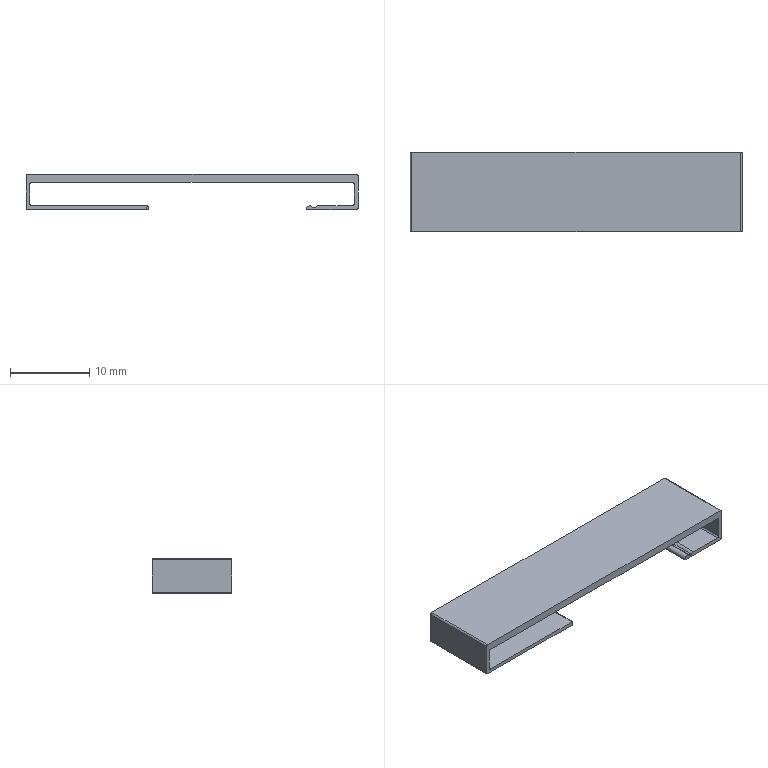Part | SolidWorks | features ICE 4, Extrusion 1, Fillet 1 | 1 solid | 30 faces | box 42 x 10 x 4.5 mm | volume 558.172 mm3 | cylinder 16 | plane 14 | commonest cylinder face diameters 0.4 x12 0.5 x2 0.8 x1 1 x1
STEP:
#1=CARTESIAN_POINT('',(-106.106,120.619,0.2323));
#2=VERTEX_POINT('',#1);
#3=CARTESIAN_POINT('',(-105.914,120.619,0.3216));
#4=VERTEX_POINT('',#3);
#5=CARTESIAN_POINT('',(-106.106,120.619,0.4823));
#6=DIRECTION('',(0.,-1.,0.));
#7=DIRECTION('',(0.,0.,-1.));
#8=AXIS2_PLACEMENT_3D('',#5,#6,#7);
#9=CIRCLE('',#8,0.25);
#10=EDGE_CURVE('',#2,#4,#9,.T.);
#11=ORIENTED_EDGE('',*,*,#10,.F.);
#12=CARTESIAN_POINT('',(-106.106,110.619,0.2323));
#13=VERTEX_POINT('',#12);
#14=CARTESIAN_POINT('',(-106.106,127.138,0.2323));
#15=DIRECTION('',(0.,-1.,0.));
#16=VECTOR('',#15,1000.);
#17=LINE('',#14,#16);
#18=EDGE_CURVE('',#2,#13,#17,.T.);
#19=ORIENTED_EDGE('',*,*,#18,.T.);
#20=CARTESIAN_POINT('',(-105.914,110.619,0.3216));
#21=VERTEX_POINT('',#20);
#22=CARTESIAN_POINT('',(-106.106,110.619,0.4823));
#23=DIRECTION('',(0.,1.,0.));
#24=DIRECTION('',(0.,0.,-1.));
#25=AXIS2_PLACEMENT_3D('',#22,#23,#24);
#26=CIRCLE('',#25,0.25);
#27=EDGE_CURVE('',#21,#13,#26,.T.);
#28=ORIENTED_EDGE('',*,*,#27,.F.);
#29=CARTESIAN_POINT('',(-105.914,127.138,0.3216));
#30=DIRECTION('',(0.,-1.,0.));
#31=VECTOR('',#30,1000.);
#32=LINE('',#29,#31);
#33=EDGE_CURVE('',#4,#21,#32,.T.);
#34=ORIENTED_EDGE('',*,*,#33,.F.);
#35=EDGE_LOOP('',(#11,#19,#28,#34));
#36=FACE_OUTER_BOUND('',#35,.T.);
#37=CARTESIAN_POINT('',(-106.106,127.138,0.4823));
#38=DIRECTION('',(0.,-1.,0.));
#39=DIRECTION('',(0.,0.,-1.));
#40=AXIS2_PLACEMENT_3D('',#37,#38,#39);
#41=CYLINDRICAL_SURFACE('',#40,0.25);
#42=ADVANCED_FACE('',(#36),#41,.F.);
#43=CARTESIAN_POINT('',(-142.531,120.619,4.3));
#44=VERTEX_POINT('',#43);
#45=CARTESIAN_POINT('',(-142.531,120.619,0.2));
#46=VERTEX_POINT('',#45);
#47=CARTESIAN_POINT('',(-142.531,120.619,0.5));
#48=DIRECTION('',(0.,0.,-1.));
#49=VECTOR('',#48,1000.);
#50=LINE('',#47,#49);
#51=EDGE_CURVE('',#44,#46,#50,.T.);
#52=ORIENTED_EDGE('',*,*,#51,.T.);
#53=CARTESIAN_POINT('',(-142.531,110.619,0.2));
#54=VERTEX_POINT('',#53);
#55=CARTESIAN_POINT('',(-142.531,120.619,0.2));
#56=DIRECTION('',(0.,-1.,0.));
#57=VECTOR('',#56,1000.);
#58=LINE('',#55,#57);
#59=EDGE_CURVE('',#46,#54,#58,.T.);
#60=ORIENTED_EDGE('',*,*,#59,.T.);
#61=CARTESIAN_POINT('',(-142.531,110.619,4.3));
#62=VERTEX_POINT('',#61);
#63=CARTESIAN_POINT('',(-142.531,110.619,0.5));
#64=DIRECTION('',(0.,0.,-1.));
#65=VECTOR('',#64,1000.);
#66=LINE('',#63,#65);
#67=EDGE_CURVE('',#62,#54,#66,.T.);
#68=ORIENTED_EDGE('',*,*,#67,.F.);
#69=CARTESIAN_POINT('',(-142.531,120.619,4.3));
#70=DIRECTION('',(0.,1.,0.));
#71=VECTOR('',#70,1000.);
#72=LINE('',#69,#71);
#73=EDGE_CURVE('',#62,#44,#72,.T.);
#74=ORIENTED_EDGE('',*,*,#73,.T.);
#75=EDGE_LOOP('',(#52,#60,#68,#74));
#76=FACE_OUTER_BOUND('',#75,.T.);
#77=CARTESIAN_POINT('',(-142.531,120.619,0.5));
#78=DIRECTION('',(1.,0.,0.));
#79=DIRECTION('',(0.,1.,0.));
#80=AXIS2_PLACEMENT_3D('',#77,#78,#79);
#81=PLANE('',#80);
#82=ADVANCED_FACE('',(#76),#81,.F.);
#83=CARTESIAN_POINT('',(-142.331,110.619,0.));
#84=VERTEX_POINT('',#83);
#85=CARTESIAN_POINT('',(-127.231,110.619,0.));
#86=VERTEX_POINT('',#85);
#87=CARTESIAN_POINT('',(-142.531,110.619,0.));
#88=DIRECTION('',(1.,0.,0.));
#89=VECTOR('',#88,1000.);
#90=LINE('',#87,#89);
#91=EDGE_CURVE('',#84,#86,#90,.T.);
#92=ORIENTED_EDGE('',*,*,#91,.T.);
#93=CARTESIAN_POINT('',(-127.231,110.619,0.5));
#94=VERTEX_POINT('',#93);
#95=CARTESIAN_POINT('',(-127.231,110.619,0.5));
#96=DIRECTION('',(0.,0.,1.));
#97=VECTOR('',#96,1000.);
#98=LINE('',#95,#97);
#99=EDGE_CURVE('',#86,#94,#98,.T.);
#100=ORIENTED_EDGE('',*,*,#99,.T.);
#101=CARTESIAN_POINT('',(-141.831,110.619,0.5));
#102=VERTEX_POINT('',#101);
#103=CARTESIAN_POINT('',(-142.531,110.619,0.5));
#104=DIRECTION('',(1.,0.,0.));
#105=VECTOR('',#104,1000.);
#106=LINE('',#103,#105);
#107=EDGE_CURVE('',#102,#94,#106,.T.);
#108=ORIENTED_EDGE('',*,*,#107,.F.);
#109=CARTESIAN_POINT('',(-142.031,110.619,0.7));
#110=VERTEX_POINT('',#109);
#111=CARTESIAN_POINT('',(-141.831,110.619,0.7));
#112=DIRECTION('',(0.,1.,0.));
#113=DIRECTION('',(0.,0.,1.));
#114=AXIS2_PLACEMENT_3D('',#111,#112,#113);
#115=CIRCLE('',#114,0.2);
#116=EDGE_CURVE('',#102,#110,#115,.T.);
#117=ORIENTED_EDGE('',*,*,#116,.T.);
#118=CARTESIAN_POINT('',(-142.031,110.619,3.3));
#119=VERTEX_POINT('',#118);
#120=CARTESIAN_POINT('',(-142.031,110.619,3.5));
#121=DIRECTION('',(0.,0.,-1.));
#122=VECTOR('',#121,1000.);
#123=LINE('',#120,#122);
#124=EDGE_CURVE('',#119,#110,#123,.T.);
#125=ORIENTED_EDGE('',*,*,#124,.F.);
#126=CARTESIAN_POINT('',(-141.831,110.619,3.5));
#127=VERTEX_POINT('',#126);
#128=CARTESIAN_POINT('',(-141.831,110.619,3.3));
#129=DIRECTION('',(0.,1.,0.));
#130=DIRECTION('',(0.,0.,1.));
#131=AXIS2_PLACEMENT_3D('',#128,#129,#130);
#132=CIRCLE('',#131,0.2);
#133=EDGE_CURVE('',#119,#127,#132,.T.);
#134=ORIENTED_EDGE('',*,*,#133,.T.);
#135=CARTESIAN_POINT('',(-101.231,110.619,3.5));
#136=VERTEX_POINT('',#135);
#137=CARTESIAN_POINT('',(-142.531,110.619,3.5));
#138=DIRECTION('',(1.,0.,0.));
#139=VECTOR('',#138,1000.);
#140=LINE('',#137,#139);
#141=EDGE_CURVE('',#127,#136,#140,.T.);
#142=ORIENTED_EDGE('',*,*,#141,.T.);
#143=CARTESIAN_POINT('',(-101.031,110.619,3.3));
#144=VERTEX_POINT('',#143);
#145=CARTESIAN_POINT('',(-101.231,110.619,3.3));
#146=DIRECTION('',(0.,1.,0.));
#147=DIRECTION('',(0.,0.,1.));
#148=AXIS2_PLACEMENT_3D('',#145,#146,#147);
#149=CIRCLE('',#148,0.2);
#150=EDGE_CURVE('',#136,#144,#149,.T.);
#151=ORIENTED_EDGE('',*,*,#150,.T.);
#152=CARTESIAN_POINT('',(-101.031,110.619,0.7));
#153=VERTEX_POINT('',#152);
#154=CARTESIAN_POINT('',(-101.031,110.619,0.));
#155=DIRECTION('',(0.,0.,1.));
#156=VECTOR('',#155,1000.);
#157=LINE('',#154,#156);
#158=EDGE_CURVE('',#153,#144,#157,.T.);
#159=ORIENTED_EDGE('',*,*,#158,.F.);
#160=CARTESIAN_POINT('',(-101.231,110.619,0.5));
#161=VERTEX_POINT('',#160);
#162=CARTESIAN_POINT('',(-101.231,110.619,0.7));
#163=DIRECTION('',(0.,1.,0.));
#164=DIRECTION('',(0.,0.,1.));
#165=AXIS2_PLACEMENT_3D('',#162,#163,#164);
#166=CIRCLE('',#165,0.2);
#167=EDGE_CURVE('',#153,#161,#166,.T.);
#168=ORIENTED_EDGE('',*,*,#167,.T.);
#169=CARTESIAN_POINT('',(-105.531,110.619,0.5));
#170=VERTEX_POINT('',#169);
#171=CARTESIAN_POINT('',(-105.531,110.619,0.5));
#172=DIRECTION('',(-1.,0.,0.));
#173=VECTOR('',#172,1000.);
#174=LINE('',#171,#173);
#175=EDGE_CURVE('',#161,#170,#174,.T.);
#176=ORIENTED_EDGE('',*,*,#175,.T.);
#177=CARTESIAN_POINT('',(-105.531,110.619,0.));
#178=DIRECTION('',(0.,-1.,0.));
#179=DIRECTION('',(0.,0.,-1.));
#180=AXIS2_PLACEMENT_3D('',#177,#178,#179);
#181=CIRCLE('',#180,0.5);
#182=EDGE_CURVE('',#170,#21,#181,.T.);
#183=ORIENTED_EDGE('',*,*,#182,.T.);
#184=ORIENTED_EDGE('',*,*,#27,.T.);
#185=CARTESIAN_POINT('',(-106.308,110.619,0.3353));
#186=VERTEX_POINT('',#185);
#187=CARTESIAN_POINT('',(-106.106,110.619,0.4823));
#188=DIRECTION('',(0.,1.,0.));
#189=DIRECTION('',(0.,0.,-1.));
#190=AXIS2_PLACEMENT_3D('',#187,#188,#189);
#191=CIRCLE('',#190,0.25);
#192=EDGE_CURVE('',#13,#186,#191,.T.);
#193=ORIENTED_EDGE('',*,*,#192,.T.);
#194=CARTESIAN_POINT('',(-107.031,110.619,0.1));
#195=VERTEX_POINT('',#194);
#196=CARTESIAN_POINT('',(-106.631,110.619,0.1));
#197=DIRECTION('',(0.,-1.,0.));
#198=DIRECTION('',(0.,0.,-1.));
#199=AXIS2_PLACEMENT_3D('',#196,#197,#198);
#200=CIRCLE('',#199,0.4);
#201=EDGE_CURVE('',#186,#195,#200,.T.);
#202=ORIENTED_EDGE('',*,*,#201,.T.);
#203=CARTESIAN_POINT('',(-107.031,110.619,0.));
#204=VERTEX_POINT('',#203);
#205=CARTESIAN_POINT('',(-107.031,110.619,0.));
#206=DIRECTION('',(0.,0.,-1.));
#207=VECTOR('',#206,1000.);
#208=LINE('',#205,#207);
#209=EDGE_CURVE('',#195,#204,#208,.T.);
#210=ORIENTED_EDGE('',*,*,#209,.T.);
#211=CARTESIAN_POINT('',(-100.731,110.619,0.));
#212=VERTEX_POINT('',#211);
#213=CARTESIAN_POINT('',(-100.531,110.619,0.));
#214=DIRECTION('',(1.,0.,0.));
#215=VECTOR('',#214,1000.);
#216=LINE('',#213,#215);
#217=EDGE_CURVE('',#204,#212,#216,.T.);
#218=ORIENTED_EDGE('',*,*,#217,.T.);
#219=CARTESIAN_POINT('',(-100.531,110.619,0.2));
#220=VERTEX_POINT('',#219);
#221=CARTESIAN_POINT('',(-100.731,110.619,0.2));
#222=DIRECTION('',(0.,-1.,0.));
#223=DIRECTION('',(0.,0.,1.));
#224=AXIS2_PLACEMENT_3D('',#221,#222,#223);
#225=CIRCLE('',#224,0.2);
#226=EDGE_CURVE('',#212,#220,#225,.T.);
#227=ORIENTED_EDGE('',*,*,#226,.T.);
#228=CARTESIAN_POINT('',(-100.531,110.619,4.3));
#229=VERTEX_POINT('',#228);
#230=CARTESIAN_POINT('',(-100.531,110.619,4.5));
#231=DIRECTION('',(0.,0.,-1.));
#232=VECTOR('',#231,1000.);
#233=LINE('',#230,#232);
#234=EDGE_CURVE('',#229,#220,#233,.T.);
#235=ORIENTED_EDGE('',*,*,#234,.F.);
#236=CARTESIAN_POINT('',(-100.731,110.619,4.5));
#237=VERTEX_POINT('',#236);
#238=CARTESIAN_POINT('',(-100.731,110.619,4.3));
#239=DIRECTION('',(0.,-1.,0.));
#240=DIRECTION('',(0.,0.,1.));
#241=AXIS2_PLACEMENT_3D('',#238,#239,#240);
#242=CIRCLE('',#241,0.2);
#243=EDGE_CURVE('',#229,#237,#242,.T.);
#244=ORIENTED_EDGE('',*,*,#243,.T.);
#245=CARTESIAN_POINT('',(-142.331,110.619,4.5));
#246=VERTEX_POINT('',#245);
#247=CARTESIAN_POINT('',(-142.531,110.619,4.5));
#248=DIRECTION('',(1.,0.,0.));
#249=VECTOR('',#248,1000.);
#250=LINE('',#247,#249);
#251=EDGE_CURVE('',#246,#237,#250,.T.);
#252=ORIENTED_EDGE('',*,*,#251,.F.);
#253=CARTESIAN_POINT('',(-142.331,110.619,4.3));
#254=DIRECTION('',(0.,-1.,0.));
#255=DIRECTION('',(0.,0.,1.));
#256=AXIS2_PLACEMENT_3D('',#253,#254,#255);
#257=CIRCLE('',#256,0.2);
#258=EDGE_CURVE('',#246,#62,#257,.T.);
#259=ORIENTED_EDGE('',*,*,#258,.T.);
#260=ORIENTED_EDGE('',*,*,#67,.T.);
#261=CARTESIAN_POINT('',(-142.331,110.619,0.2));
#262=DIRECTION('',(0.,-1.,0.));
#263=DIRECTION('',(0.,0.,1.));
#264=AXIS2_PLACEMENT_3D('',#261,#262,#263);
#265=CIRCLE('',#264,0.2);
#266=EDGE_CURVE('',#54,#84,#265,.T.);
#267=ORIENTED_EDGE('',*,*,#266,.T.);
#268=EDGE_LOOP('',(#92,#100,#108,#117,#125,#134,#142,#151,#159,#168,#176,#183,#184,#193,#202,#210,#218,#227,#235,#244,#252,#259,#260,#267));
#269=FACE_OUTER_BOUND('',#268,.T.);
#270=CARTESIAN_POINT('',(-142.531,110.619,0.5));
#271=DIRECTION('',(0.,1.,0.));
#272=DIRECTION('',(0.,0.,1.));
#273=AXIS2_PLACEMENT_3D('',#270,#271,#272);
#274=PLANE('',#273);
#275=ADVANCED_FACE('',(#269),#274,.F.);
#276=CARTESIAN_POINT('',(-127.031,120.419,0.3));
#277=VERTEX_POINT('',#276);
#278=CARTESIAN_POINT('',(-127.031,110.819,0.3));
#279=VERTEX_POINT('',#278);
#280=CARTESIAN_POINT('',(-127.031,110.619,0.3));
#281=DIRECTION('',(0.,-1.,0.));
#282=VECTOR('',#281,1000.);
#283=LINE('',#280,#282);
#284=EDGE_CURVE('',#277,#279,#283,.T.);
#285=ORIENTED_EDGE('',*,*,#284,.T.);
#286=CARTESIAN_POINT('',(-127.031,110.819,0.2));
#287=VERTEX_POINT('',#286);
#288=CARTESIAN_POINT('',(-127.031,110.819,0.5));
#289=DIRECTION('',(0.,0.,-1.));
#290=VECTOR('',#289,1000.);
#291=LINE('',#288,#290);
#292=EDGE_CURVE('',#279,#287,#291,.T.);
#293=ORIENTED_EDGE('',*,*,#292,.T.);
#294=CARTESIAN_POINT('',(-127.031,120.419,0.2));
#295=VERTEX_POINT('',#294);
#296=CARTESIAN_POINT('',(-127.031,120.619,0.2));
#297=DIRECTION('',(0.,1.,0.));
#298=VECTOR('',#297,1000.);
#299=LINE('',#296,#298);
#300=EDGE_CURVE('',#287,#295,#299,.T.);
#301=ORIENTED_EDGE('',*,*,#300,.T.);
#302=CARTESIAN_POINT('',(-127.031,120.419,0.5));
#303=DIRECTION('',(0.,0.,1.));
#304=VECTOR('',#303,1000.);
#305=LINE('',#302,#304);
#306=EDGE_CURVE('',#295,#277,#305,.T.);
#307=ORIENTED_EDGE('',*,*,#306,.T.);
#308=EDGE_LOOP('',(#285,#293,#301,#307));
#309=FACE_OUTER_BOUND('',#308,.T.);
#310=CARTESIAN_POINT('',(-127.031,120.619,0.5));
#311=DIRECTION('',(-1.,0.,0.));
#312=DIRECTION('',(0.,0.,1.));
#313=AXIS2_PLACEMENT_3D('',#310,#311,#312);
#314=PLANE('',#313);
#315=ADVANCED_FACE('',(#309),#314,.F.);
#316=CARTESIAN_POINT('',(-127.231,120.619,0.5));
#317=VERTEX_POINT('',#316);
#318=CARTESIAN_POINT('',(-141.831,120.619,0.5));
#319=VERTEX_POINT('',#318);
#320=CARTESIAN_POINT('',(-142.531,120.619,0.5));
#321=DIRECTION('',(-1.,0.,0.));
#322=VECTOR('',#321,1000.);
#323=LINE('',#320,#322);
#324=EDGE_CURVE('',#317,#319,#323,.T.);
#325=ORIENTED_EDGE('',*,*,#324,.F.);
#326=CARTESIAN_POINT('',(-127.231,120.619,0.));
#327=VERTEX_POINT('',#326);
#328=CARTESIAN_POINT('',(-127.231,120.619,0.5));
#329=DIRECTION('',(0.,0.,-1.));
#330=VECTOR('',#329,1000.);
#331=LINE('',#328,#330);
#332=EDGE_CURVE('',#317,#327,#331,.T.);
#333=ORIENTED_EDGE('',*,*,#332,.T.);
#334=CARTESIAN_POINT('',(-142.331,120.619,0.));
#335=VERTEX_POINT('',#334);
#336=CARTESIAN_POINT('',(-142.531,120.619,0.));
#337=DIRECTION('',(-1.,0.,0.));
#338=VECTOR('',#337,1000.);
#339=LINE('',#336,#338);
#340=EDGE_CURVE('',#327,#335,#339,.T.);
#341=ORIENTED_EDGE('',*,*,#340,.T.);
#342=CARTESIAN_POINT('',(-142.331,120.619,0.2));
#343=DIRECTION('',(0.,1.,0.));
#344=DIRECTION('',(0.,0.,-1.));
#345=AXIS2_PLACEMENT_3D('',#342,#343,#344);
#346=CIRCLE('',#345,0.2);
#347=EDGE_CURVE('',#335,#46,#346,.T.);
#348=ORIENTED_EDGE('',*,*,#347,.T.);
#349=ORIENTED_EDGE('',*,*,#51,.F.);
#350=CARTESIAN_POINT('',(-142.331,120.619,4.5));
#351=VERTEX_POINT('',#350);
#352=CARTESIAN_POINT('',(-142.331,120.619,4.3));
#353=DIRECTION('',(0.,1.,0.));
#354=DIRECTION('',(0.,0.,-1.));
#355=AXIS2_PLACEMENT_3D('',#352,#353,#354);
#356=CIRCLE('',#355,0.2);
#357=EDGE_CURVE('',#44,#351,#356,.T.);
#358=ORIENTED_EDGE('',*,*,#357,.T.);
#359=CARTESIAN_POINT('',(-100.731,120.619,4.5));
#360=VERTEX_POINT('',#359);
#361=CARTESIAN_POINT('',(-142.531,120.619,4.5));
#362=DIRECTION('',(-1.,0.,0.));
#363=VECTOR('',#362,1000.);
#364=LINE('',#361,#363);
#365=EDGE_CURVE('',#360,#351,#364,.T.);
#366=ORIENTED_EDGE('',*,*,#365,.F.);
#367=CARTESIAN_POINT('',(-100.531,120.619,4.3));
#368=VERTEX_POINT('',#367);
#369=CARTESIAN_POINT('',(-100.731,120.619,4.3));
#370=DIRECTION('',(0.,1.,0.));
#371=DIRECTION('',(0.,0.,-1.));
#372=AXIS2_PLACEMENT_3D('',#369,#370,#371);
#373=CIRCLE('',#372,0.2);
#374=EDGE_CURVE('',#360,#368,#373,.T.);
#375=ORIENTED_EDGE('',*,*,#374,.T.);
#376=CARTESIAN_POINT('',(-100.531,120.619,0.2));
#377=VERTEX_POINT('',#376);
#378=CARTESIAN_POINT('',(-100.531,120.619,4.5));
#379=DIRECTION('',(0.,0.,-1.));
#380=VECTOR('',#379,1000.);
#381=LINE('',#378,#380);
#382=EDGE_CURVE('',#368,#377,#381,.T.);
#383=ORIENTED_EDGE('',*,*,#382,.T.);
#384=CARTESIAN_POINT('',(-100.731,120.619,0.));
#385=VERTEX_POINT('',#384);
#386=CARTESIAN_POINT('',(-100.731,120.619,0.2));
#387=DIRECTION('',(0.,1.,0.));
#388=DIRECTION('',(0.,0.,-1.));
#389=AXIS2_PLACEMENT_3D('',#386,#387,#388);
#390=CIRCLE('',#389,0.2);
#391=EDGE_CURVE('',#377,#385,#390,.T.);
#392=ORIENTED_EDGE('',*,*,#391,.T.);
#393=CARTESIAN_POINT('',(-107.031,120.619,0.));
#394=VERTEX_POINT('',#393);
#395=CARTESIAN_POINT('',(-100.531,120.619,0.));
#396=DIRECTION('',(-1.,0.,0.));
#397=VECTOR('',#396,1000.);
#398=LINE('',#395,#397);
#399=EDGE_CURVE('',#385,#394,#398,.T.);
#400=ORIENTED_EDGE('',*,*,#399,.T.);
#401=CARTESIAN_POINT('',(-107.031,120.619,0.1));
#402=VERTEX_POINT('',#401);
#403=CARTESIAN_POINT('',(-107.031,120.619,0.));
#404=DIRECTION('',(0.,0.,1.));
#405=VECTOR('',#404,1000.);
#406=LINE('',#403,#405);
#407=EDGE_CURVE('',#394,#402,#406,.T.);
#408=ORIENTED_EDGE('',*,*,#407,.T.);
#409=CARTESIAN_POINT('',(-106.308,120.619,0.3353));
#410=VERTEX_POINT('',#409);
#411=CARTESIAN_POINT('',(-106.631,120.619,0.1));
#412=DIRECTION('',(0.,1.,0.));
#413=DIRECTION('',(0.,0.,-1.));
#414=AXIS2_PLACEMENT_3D('',#411,#412,#413);
#415=CIRCLE('',#414,0.4);
#416=EDGE_CURVE('',#402,#410,#415,.T.);
#417=ORIENTED_EDGE('',*,*,#416,.T.);
#418=CARTESIAN_POINT('',(-106.106,120.619,0.4823));
#419=DIRECTION('',(0.,-1.,0.));
#420=DIRECTION('',(0.,0.,-1.));
#421=AXIS2_PLACEMENT_3D('',#418,#419,#420);
#422=CIRCLE('',#421,0.25);
#423=EDGE_CURVE('',#410,#2,#422,.T.);
#424=ORIENTED_EDGE('',*,*,#423,.T.);
#425=ORIENTED_EDGE('',*,*,#10,.T.);
#426=CARTESIAN_POINT('',(-105.531,120.619,0.5));
#427=VERTEX_POINT('',#426);
#428=CARTESIAN_POINT('',(-105.531,120.619,0.));
#429=DIRECTION('',(0.,1.,0.));
#430=DIRECTION('',(0.,0.,-1.));
#431=AXIS2_PLACEMENT_3D('',#428,#429,#430);
#432=CIRCLE('',#431,0.5);
#433=EDGE_CURVE('',#4,#427,#432,.T.);
#434=ORIENTED_EDGE('',*,*,#433,.T.);
#435=CARTESIAN_POINT('',(-101.231,120.619,0.5));
#436=VERTEX_POINT('',#435);
#437=CARTESIAN_POINT('',(-105.531,120.619,0.5));
#438=DIRECTION('',(1.,0.,0.));
#439=VECTOR('',#438,1000.);
#440=LINE('',#437,#439);
#441=EDGE_CURVE('',#427,#436,#440,.T.);
#442=ORIENTED_EDGE('',*,*,#441,.T.);
#443=CARTESIAN_POINT('',(-101.031,120.619,0.7));
#444=VERTEX_POINT('',#443);
#445=CARTESIAN_POINT('',(-101.231,120.619,0.7));
#446=DIRECTION('',(0.,-1.,0.));
#447=DIRECTION('',(0.,0.,-1.));
#448=AXIS2_PLACEMENT_3D('',#445,#446,#447);
#449=CIRCLE('',#448,0.2);
#450=EDGE_CURVE('',#436,#444,#449,.T.);
#451=ORIENTED_EDGE('',*,*,#450,.T.);
#452=CARTESIAN_POINT('',(-101.031,120.619,3.3));
#453=VERTEX_POINT('',#452);
#454=CARTESIAN_POINT('',(-101.031,120.619,0.));
#455=DIRECTION('',(0.,0.,1.));
#456=VECTOR('',#455,1000.);
#457=LINE('',#454,#456);
#458=EDGE_CURVE('',#444,#453,#457,.T.);
#459=ORIENTED_EDGE('',*,*,#458,.T.);
#460=CARTESIAN_POINT('',(-101.231,120.619,3.5));
#461=VERTEX_POINT('',#460);
#462=CARTESIAN_POINT('',(-101.231,120.619,3.3));
#463=DIRECTION('',(0.,-1.,0.));
#464=DIRECTION('',(0.,0.,-1.));
#465=AXIS2_PLACEMENT_3D('',#462,#463,#464);
#466=CIRCLE('',#465,0.2);
#467=EDGE_CURVE('',#453,#461,#466,.T.);
#468=ORIENTED_EDGE('',*,*,#467,.T.);
#469=CARTESIAN_POINT('',(-141.831,120.619,3.5));
#470=VERTEX_POINT('',#469);
#471=CARTESIAN_POINT('',(-142.531,120.619,3.5));
#472=DIRECTION('',(-1.,0.,0.));
#473=VECTOR('',#472,1000.);
#474=LINE('',#471,#473);
#475=EDGE_CURVE('',#461,#470,#474,.T.);
#476=ORIENTED_EDGE('',*,*,#475,.T.);
#477=CARTESIAN_POINT('',(-142.031,120.619,3.3));
#478=VERTEX_POINT('',#477);
#479=CARTESIAN_POINT('',(-141.831,120.619,3.3));
#480=DIRECTION('',(0.,-1.,0.));
#481=DIRECTION('',(0.,0.,-1.));
#482=AXIS2_PLACEMENT_3D('',#479,#480,#481);
#483=CIRCLE('',#482,0.2);
#484=EDGE_CURVE('',#470,#478,#483,.T.);
#485=ORIENTED_EDGE('',*,*,#484,.T.);
#486=CARTESIAN_POINT('',(-142.031,120.619,0.7));
#487=VERTEX_POINT('',#486);
#488=CARTESIAN_POINT('',(-142.031,120.619,3.5));
#489=DIRECTION('',(0.,0.,-1.));
#490=VECTOR('',#489,1000.);
#491=LINE('',#488,#490);
#492=EDGE_CURVE('',#478,#487,#491,.T.);
#493=ORIENTED_EDGE('',*,*,#492,.T.);
#494=CARTESIAN_POINT('',(-141.831,120.619,0.7));
#495=DIRECTION('',(0.,-1.,0.));
#496=DIRECTION('',(0.,0.,-1.));
#497=AXIS2_PLACEMENT_3D('',#494,#495,#496);
#498=CIRCLE('',#497,0.2);
#499=EDGE_CURVE('',#487,#319,#498,.T.);
#500=ORIENTED_EDGE('',*,*,#499,.T.);
#501=EDGE_LOOP('',(#325,#333,#341,#348,#349,#358,#366,#375,#383,#392,#400,#408,#417,#424,#425,#434,#442,#451,#459,#468,#476,#485,#493,#500));
#502=FACE_OUTER_BOUND('',#501,.T.);
#503=CARTESIAN_POINT('',(-142.531,120.619,0.5));
#504=DIRECTION('',(0.,-1.,0.));
#505=DIRECTION('',(0.,0.,-1.));
#506=AXIS2_PLACEMENT_3D('',#503,#504,#505);
#507=PLANE('',#506);
#508=ADVANCED_FACE('',(#502),#507,.F.);
#509=ORIENTED_EDGE('',*,*,#107,.T.);
#510=CARTESIAN_POINT('',(-127.231,120.619,0.5));
#511=DIRECTION('',(0.,1.,0.));
#512=VECTOR('',#511,1000.);
#513=LINE('',#510,#512);
#514=EDGE_CURVE('',#94,#317,#513,.T.);
#515=ORIENTED_EDGE('',*,*,#514,.T.);
#516=ORIENTED_EDGE('',*,*,#324,.T.);
#517=CARTESIAN_POINT('',(-141.831,0.,0.5));
#518=DIRECTION('',(0.,-1.,0.));
#519=VECTOR('',#518,1000.);
#520=LINE('',#517,#519);
#521=EDGE_CURVE('',#319,#102,#520,.T.);
#522=ORIENTED_EDGE('',*,*,#521,.T.);
#523=EDGE_LOOP('',(#509,#515,#516,#522));
#524=FACE_OUTER_BOUND('',#523,.T.);
#525=CARTESIAN_POINT('',(0.,0.,0.5));
#526=DIRECTION('',(0.,0.,1.));
#527=DIRECTION('',(1.,0.,0.));
#528=AXIS2_PLACEMENT_3D('',#525,#526,#527);
#529=PLANE('',#528);
#530=ADVANCED_FACE('',(#524),#529,.T.);
#531=ORIENTED_EDGE('',*,*,#340,.F.);
#532=CARTESIAN_POINT('',(-127.231,0.,0.));
#533=DIRECTION('',(0.,-1.,0.));
#534=VECTOR('',#533,1000.);
#535=LINE('',#532,#534);
#536=EDGE_CURVE('',#327,#86,#535,.T.);
#537=ORIENTED_EDGE('',*,*,#536,.T.);
#538=ORIENTED_EDGE('',*,*,#91,.F.);
#539=CARTESIAN_POINT('',(-142.331,0.,0.));
#540=DIRECTION('',(0.,1.,0.));
#541=VECTOR('',#540,1000.);
#542=LINE('',#539,#541);
#543=EDGE_CURVE('',#84,#335,#542,.T.);
#544=ORIENTED_EDGE('',*,*,#543,.T.);
#545=EDGE_LOOP('',(#531,#537,#538,#544));
#546=FACE_OUTER_BOUND('',#545,.T.);
#547=CARTESIAN_POINT('',(0.,0.,0.));
#548=DIRECTION('',(0.,0.,1.));
#549=DIRECTION('',(1.,0.,0.));
#550=AXIS2_PLACEMENT_3D('',#547,#548,#549);
#551=PLANE('',#550);
#552=ADVANCED_FACE('',(#546),#551,.F.);
#553=ORIENTED_EDGE('',*,*,#124,.T.);
#554=CARTESIAN_POINT('',(-142.031,120.619,0.7));
#555=DIRECTION('',(0.,1.,0.));
#556=VECTOR('',#555,1000.);
#557=LINE('',#554,#556);
#558=EDGE_CURVE('',#110,#487,#557,.T.);
#559=ORIENTED_EDGE('',*,*,#558,.T.);
#560=ORIENTED_EDGE('',*,*,#492,.F.);
#561=CARTESIAN_POINT('',(-142.031,110.619,3.3));
#562=DIRECTION('',(0.,-1.,0.));
#563=VECTOR('',#562,1000.);
#564=LINE('',#561,#563);
#565=EDGE_CURVE('',#478,#119,#564,.T.);
#566=ORIENTED_EDGE('',*,*,#565,.T.);
#567=EDGE_LOOP('',(#553,#559,#560,#566));
#568=FACE_OUTER_BOUND('',#567,.T.);
#569=CARTESIAN_POINT('',(-142.031,120.619,3.5));
#570=DIRECTION('',(-1.,0.,0.));
#571=DIRECTION('',(0.,-1.,0.));
#572=AXIS2_PLACEMENT_3D('',#569,#570,#571);
#573=PLANE('',#572);
#574=ADVANCED_FACE('',(#568),#573,.F.);
#575=ORIENTED_EDGE('',*,*,#475,.F.);
#576=CARTESIAN_POINT('',(-101.231,0.,3.5));
#577=DIRECTION('',(0.,-1.,0.));
#578=VECTOR('',#577,1000.);
#579=LINE('',#576,#578);
#580=EDGE_CURVE('',#461,#136,#579,.T.);
#581=ORIENTED_EDGE('',*,*,#580,.T.);
#582=ORIENTED_EDGE('',*,*,#141,.F.);
#583=CARTESIAN_POINT('',(-141.831,120.619,3.5));
#584=DIRECTION('',(0.,1.,0.));
#585=VECTOR('',#584,1000.);
#586=LINE('',#583,#585);
#587=EDGE_CURVE('',#127,#470,#586,.T.);
#588=ORIENTED_EDGE('',*,*,#587,.T.);
#589=EDGE_LOOP('',(#575,#581,#582,#588));
#590=FACE_OUTER_BOUND('',#589,.T.);
#591=CARTESIAN_POINT('',(0.,0.,3.5));
#592=DIRECTION('',(0.,0.,1.));
#593=DIRECTION('',(1.,0.,0.));
#594=AXIS2_PLACEMENT_3D('',#591,#592,#593);
#595=PLANE('',#594);
#596=ADVANCED_FACE('',(#590),#595,.F.);
#597=ORIENTED_EDGE('',*,*,#234,.T.);
#598=CARTESIAN_POINT('',(-100.531,120.619,0.2));
#599=DIRECTION('',(0.,1.,0.));
#600=VECTOR('',#599,1000.);
#601=LINE('',#598,#600);
#602=EDGE_CURVE('',#220,#377,#601,.T.);
#603=ORIENTED_EDGE('',*,*,#602,.T.);
#604=ORIENTED_EDGE('',*,*,#382,.F.);
#605=CARTESIAN_POINT('',(-100.531,110.619,4.3));
#606=DIRECTION('',(0.,-1.,0.));
#607=VECTOR('',#606,1000.);
#608=LINE('',#605,#607);
#609=EDGE_CURVE('',#368,#229,#608,.T.);
#610=ORIENTED_EDGE('',*,*,#609,.T.);
#611=EDGE_LOOP('',(#597,#603,#604,#610));
#612=FACE_OUTER_BOUND('',#611,.T.);
#613=CARTESIAN_POINT('',(-100.531,120.619,4.5));
#614=DIRECTION('',(-1.,0.,0.));
#615=DIRECTION('',(0.,0.,1.));
#616=AXIS2_PLACEMENT_3D('',#613,#614,#615);
#617=PLANE('',#616);
#618=ADVANCED_FACE('',(#612),#617,.F.);
#619=ORIENTED_EDGE('',*,*,#251,.T.);
#620=CARTESIAN_POINT('',(-100.731,120.619,4.5));
#621=DIRECTION('',(0.,1.,0.));
#622=VECTOR('',#621,1000.);
#623=LINE('',#620,#622);
#624=EDGE_CURVE('',#237,#360,#623,.T.);
#625=ORIENTED_EDGE('',*,*,#624,.T.);
#626=ORIENTED_EDGE('',*,*,#365,.T.);
#627=CARTESIAN_POINT('',(-142.331,110.619,4.5));
#628=DIRECTION('',(0.,-1.,0.));
#629=VECTOR('',#628,1000.);
#630=LINE('',#627,#629);
#631=EDGE_CURVE('',#351,#246,#630,.T.);
#632=ORIENTED_EDGE('',*,*,#631,.T.);
#633=EDGE_LOOP('',(#619,#625,#626,#632));
#634=FACE_OUTER_BOUND('',#633,.T.);
#635=CARTESIAN_POINT('',(0.,0.,4.5));
#636=DIRECTION('',(0.,0.,1.));
#637=DIRECTION('',(1.,0.,0.));
#638=AXIS2_PLACEMENT_3D('',#635,#636,#637);
#639=PLANE('',#638);
#640=ADVANCED_FACE('',(#634),#639,.T.);
#641=ORIENTED_EDGE('',*,*,#458,.F.);
#642=CARTESIAN_POINT('',(-101.031,110.619,0.7));
#643=DIRECTION('',(0.,-1.,0.));
#644=VECTOR('',#643,1000.);
#645=LINE('',#642,#644);
#646=EDGE_CURVE('',#444,#153,#645,.T.);
#647=ORIENTED_EDGE('',*,*,#646,.T.);
#648=ORIENTED_EDGE('',*,*,#158,.T.);
#649=CARTESIAN_POINT('',(-101.031,120.619,3.3));
#650=DIRECTION('',(0.,1.,0.));
#651=VECTOR('',#650,1000.);
#652=LINE('',#649,#651);
#653=EDGE_CURVE('',#144,#453,#652,.T.);
#654=ORIENTED_EDGE('',*,*,#653,.T.);
#655=EDGE_LOOP('',(#641,#647,#648,#654));
#656=FACE_OUTER_BOUND('',#655,.T.);
#657=CARTESIAN_POINT('',(-101.031,120.619,0.));
#658=DIRECTION('',(-1.,0.,0.));
#659=DIRECTION('',(0.,-1.,0.));
#660=AXIS2_PLACEMENT_3D('',#657,#658,#659);
#661=PLANE('',#660);
#662=ADVANCED_FACE('',(#656),#661,.T.);
#663=ORIENTED_EDGE('',*,*,#399,.F.);
#664=CARTESIAN_POINT('',(-100.731,110.619,0.));
#665=DIRECTION('',(0.,-1.,0.));
#666=VECTOR('',#665,1000.);
#667=LINE('',#664,#666);
#668=EDGE_CURVE('',#385,#212,#667,.T.);
#669=ORIENTED_EDGE('',*,*,#668,.T.);
#670=ORIENTED_EDGE('',*,*,#217,.F.);
#671=CARTESIAN_POINT('',(-107.031,127.138,0.));
#672=DIRECTION('',(0.,-1.,0.));
#673=VECTOR('',#672,1000.);
#674=LINE('',#671,#673);
#675=EDGE_CURVE('',#394,#204,#674,.T.);
#676=ORIENTED_EDGE('',*,*,#675,.F.);
#677=EDGE_LOOP('',(#663,#669,#670,#676));
#678=FACE_OUTER_BOUND('',#677,.T.);
#679=CARTESIAN_POINT('',(0.,0.,0.));
#680=DIRECTION('',(0.,0.,-1.));
#681=DIRECTION('',(-1.,0.,0.));
#682=AXIS2_PLACEMENT_3D('',#679,#680,#681);
#683=PLANE('',#682);
#684=ADVANCED_FACE('',(#678),#683,.T.);
#685=ORIENTED_EDGE('',*,*,#407,.F.);
#686=ORIENTED_EDGE('',*,*,#675,.T.);
#687=ORIENTED_EDGE('',*,*,#209,.F.);
#688=CARTESIAN_POINT('',(-107.031,127.138,0.1));
#689=DIRECTION('',(0.,-1.,0.));
#690=VECTOR('',#689,1000.);
#691=LINE('',#688,#690);
#692=EDGE_CURVE('',#402,#195,#691,.T.);
#693=ORIENTED_EDGE('',*,*,#692,.F.);
#694=EDGE_LOOP('',(#685,#686,#687,#693));
#695=FACE_OUTER_BOUND('',#694,.T.);
#696=CARTESIAN_POINT('',(-107.031,127.138,0.));
#697=DIRECTION('',(-1.,0.,0.));
#698=DIRECTION('',(0.,0.,1.));
#699=AXIS2_PLACEMENT_3D('',#696,#697,#698);
#700=PLANE('',#699);
#701=ADVANCED_FACE('',(#695),#700,.T.);
#702=ORIENTED_EDGE('',*,*,#416,.F.);
#703=ORIENTED_EDGE('',*,*,#692,.T.);
#704=ORIENTED_EDGE('',*,*,#201,.F.);
#705=CARTESIAN_POINT('',(-106.308,127.138,0.3353));
#706=DIRECTION('',(0.,-1.,0.));
#707=VECTOR('',#706,1000.);
#708=LINE('',#705,#707);
#709=EDGE_CURVE('',#410,#186,#708,.T.);
#710=ORIENTED_EDGE('',*,*,#709,.F.);
#711=EDGE_LOOP('',(#702,#703,#704,#710));
#712=FACE_OUTER_BOUND('',#711,.T.);
#713=CARTESIAN_POINT('',(-106.631,127.138,0.1));
#714=DIRECTION('',(0.,-1.,0.));
#715=DIRECTION('',(0.,0.,-1.));
#716=AXIS2_PLACEMENT_3D('',#713,#714,#715);
#717=CYLINDRICAL_SURFACE('',#716,0.4);
#718=ADVANCED_FACE('',(#712),#717,.T.);
#719=ORIENTED_EDGE('',*,*,#18,.F.);
#720=ORIENTED_EDGE('',*,*,#423,.F.);
#721=ORIENTED_EDGE('',*,*,#709,.T.);
#722=ORIENTED_EDGE('',*,*,#192,.F.);
#723=EDGE_LOOP('',(#719,#720,#721,#722));
#724=FACE_OUTER_BOUND('',#723,.T.);
#725=CARTESIAN_POINT('',(-106.106,127.138,0.4823));
#726=DIRECTION('',(0.,-1.,0.));
#727=DIRECTION('',(0.,0.,-1.));
#728=AXIS2_PLACEMENT_3D('',#725,#726,#727);
#729=CYLINDRICAL_SURFACE('',#728,0.25);
#730=ADVANCED_FACE('',(#724),#729,.F.);
#731=ORIENTED_EDGE('',*,*,#433,.F.);
#732=ORIENTED_EDGE('',*,*,#33,.T.);
#733=ORIENTED_EDGE('',*,*,#182,.F.);
#734=CARTESIAN_POINT('',(-105.531,127.138,0.5));
#735=DIRECTION('',(0.,-1.,0.));
#736=VECTOR('',#735,1000.);
#737=LINE('',#734,#736);
#738=EDGE_CURVE('',#427,#170,#737,.T.);
#739=ORIENTED_EDGE('',*,*,#738,.F.);
#740=EDGE_LOOP('',(#731,#732,#733,#739));
#741=FACE_OUTER_BOUND('',#740,.T.);
#742=CARTESIAN_POINT('',(-105.531,127.138,0.));
#743=DIRECTION('',(0.,-1.,0.));
#744=DIRECTION('',(0.,0.,-1.));
#745=AXIS2_PLACEMENT_3D('',#742,#743,#744);
#746=CYLINDRICAL_SURFACE('',#745,0.5);
#747=ADVANCED_FACE('',(#741),#746,.T.);
#748=ORIENTED_EDGE('',*,*,#175,.F.);
#749=CARTESIAN_POINT('',(-101.231,120.619,0.5));
#750=DIRECTION('',(0.,1.,0.));
#751=VECTOR('',#750,1000.);
#752=LINE('',#749,#751);
#753=EDGE_CURVE('',#161,#436,#752,.T.);
#754=ORIENTED_EDGE('',*,*,#753,.T.);
#755=ORIENTED_EDGE('',*,*,#441,.F.);
#756=ORIENTED_EDGE('',*,*,#738,.T.);
#757=EDGE_LOOP('',(#748,#754,#755,#756));
#758=FACE_OUTER_BOUND('',#757,.T.);
#759=CARTESIAN_POINT('',(-105.531,127.138,0.5));
#760=DIRECTION('',(0.,0.,1.));
#761=DIRECTION('',(1.,0.,0.));
#762=AXIS2_PLACEMENT_3D('',#759,#760,#761);
#763=PLANE('',#762);
#764=ADVANCED_FACE('',(#758),#763,.T.);
#765=CARTESIAN_POINT('',(-127.231,120.619,0.));
#766=CARTESIAN_POINT('',(-127.114,120.619,0.));
#767=CARTESIAN_POINT('',(-127.031,120.536,0.08284));
#768=CARTESIAN_POINT('',(-127.031,120.419,0.2));
#769=(BOUNDED_CURVE()B_SPLINE_CURVE(3,(#765,#766,#767,#768),.UNSPECIFIED.,.F.,.F.)B_SPLINE_CURVE_WITH_KNOTS((4,4),(0.,1.571),.UNSPECIFIED.)CURVE()GEOMETRIC_REPRESENTATION_ITEM()RATIONAL_B_SPLINE_CURVE((1.,0.8047,0.8047,1.))REPRESENTATION_ITEM(''));
#770=EDGE_CURVE('',#327,#295,#769,.T.);
#771=ORIENTED_EDGE('',*,*,#770,.F.);
#772=ORIENTED_EDGE('',*,*,#332,.F.);
#773=CARTESIAN_POINT('',(-127.031,120.419,0.3));
#774=CARTESIAN_POINT('',(-127.031,120.536,0.4172));
#775=CARTESIAN_POINT('',(-127.114,120.619,0.5));
#776=CARTESIAN_POINT('',(-127.231,120.619,0.5));
#777=(BOUNDED_CURVE()B_SPLINE_CURVE(3,(#773,#774,#775,#776),.UNSPECIFIED.,.F.,.F.)B_SPLINE_CURVE_WITH_KNOTS((4,4),(1.571,3.142),.UNSPECIFIED.)CURVE()GEOMETRIC_REPRESENTATION_ITEM()RATIONAL_B_SPLINE_CURVE((1.,0.8047,0.8047,1.))REPRESENTATION_ITEM(''));
#778=EDGE_CURVE('',#277,#317,#777,.T.);
#779=ORIENTED_EDGE('',*,*,#778,.F.);
#780=ORIENTED_EDGE('',*,*,#306,.F.);
#781=EDGE_LOOP('',(#771,#772,#779,#780));
#782=FACE_OUTER_BOUND('',#781,.T.);
#783=CARTESIAN_POINT('',(-127.231,120.419,0.5));
#784=DIRECTION('',(0.,0.,-1.));
#785=DIRECTION('',(-1.,0.,0.));
#786=AXIS2_PLACEMENT_3D('',#783,#784,#785);
#787=CYLINDRICAL_SURFACE('',#786,0.2);
#788=ADVANCED_FACE('',(#782),#787,.T.);
#789=ORIENTED_EDGE('',*,*,#778,.T.);
#790=ORIENTED_EDGE('',*,*,#514,.F.);
#791=CARTESIAN_POINT('',(-127.031,110.819,0.3));
#792=CARTESIAN_POINT('',(-127.031,110.702,0.4172));
#793=CARTESIAN_POINT('',(-127.114,110.619,0.5));
#794=CARTESIAN_POINT('',(-127.231,110.619,0.5));
#795=(BOUNDED_CURVE()B_SPLINE_CURVE(3,(#791,#792,#793,#794),.UNSPECIFIED.,.F.,.F.)B_SPLINE_CURVE_WITH_KNOTS((4,4),(4.712,6.283),.UNSPECIFIED.)CURVE()GEOMETRIC_REPRESENTATION_ITEM()RATIONAL_B_SPLINE_CURVE((1.,0.8047,0.8047,1.))REPRESENTATION_ITEM(''));
#796=EDGE_CURVE('',#279,#94,#795,.T.);
#797=ORIENTED_EDGE('',*,*,#796,.F.);
#798=ORIENTED_EDGE('',*,*,#284,.F.);
#799=EDGE_LOOP('',(#789,#790,#797,#798));
#800=FACE_OUTER_BOUND('',#799,.T.);
#801=CARTESIAN_POINT('',(-127.231,0.,0.3));
#802=DIRECTION('',(0.,-1.,0.));
#803=DIRECTION('',(0.,0.,-1.));
#804=AXIS2_PLACEMENT_3D('',#801,#802,#803);
#805=CYLINDRICAL_SURFACE('',#804,0.2);
#806=ADVANCED_FACE('',(#800),#805,.T.);
#807=ORIENTED_EDGE('',*,*,#770,.T.);
#808=ORIENTED_EDGE('',*,*,#300,.F.);
#809=CARTESIAN_POINT('',(-127.231,110.619,0.));
#810=CARTESIAN_POINT('',(-127.114,110.619,0.));
#811=CARTESIAN_POINT('',(-127.031,110.702,0.08284));
#812=CARTESIAN_POINT('',(-127.031,110.819,0.2));
#813=(BOUNDED_CURVE()B_SPLINE_CURVE(3,(#809,#810,#811,#812),.UNSPECIFIED.,.F.,.T.)B_SPLINE_CURVE_WITH_KNOTS((4,4),(3.142,4.712),.UNSPECIFIED.)CURVE()GEOMETRIC_REPRESENTATION_ITEM()RATIONAL_B_SPLINE_CURVE((1.,0.8047,0.8047,1.))REPRESENTATION_ITEM(''));
#814=EDGE_CURVE('',#86,#287,#813,.T.);
#815=ORIENTED_EDGE('',*,*,#814,.F.);
#816=ORIENTED_EDGE('',*,*,#536,.F.);
#817=EDGE_LOOP('',(#807,#808,#815,#816));
#818=FACE_OUTER_BOUND('',#817,.T.);
#819=CARTESIAN_POINT('',(-127.231,120.619,0.2));
#820=DIRECTION('',(0.,1.,0.));
#821=DIRECTION('',(0.,0.,1.));
#822=AXIS2_PLACEMENT_3D('',#819,#820,#821);
#823=CYLINDRICAL_SURFACE('',#822,0.2);
#824=ADVANCED_FACE('',(#818),#823,.T.);
#825=ORIENTED_EDGE('',*,*,#796,.T.);
#826=ORIENTED_EDGE('',*,*,#99,.F.);
#827=ORIENTED_EDGE('',*,*,#814,.T.);
#828=ORIENTED_EDGE('',*,*,#292,.F.);
#829=EDGE_LOOP('',(#825,#826,#827,#828));
#830=FACE_OUTER_BOUND('',#829,.T.);
#831=CARTESIAN_POINT('',(-127.231,110.819,0.5));
#832=DIRECTION('',(0.,0.,-1.));
#833=DIRECTION('',(-1.,0.,0.));
#834=AXIS2_PLACEMENT_3D('',#831,#832,#833);
#835=CYLINDRICAL_SURFACE('',#834,0.2);
#836=ADVANCED_FACE('',(#830),#835,.T.);
#837=ORIENTED_EDGE('',*,*,#167,.F.);
#838=ORIENTED_EDGE('',*,*,#646,.F.);
#839=ORIENTED_EDGE('',*,*,#450,.F.);
#840=ORIENTED_EDGE('',*,*,#753,.F.);
#841=EDGE_LOOP('',(#837,#838,#839,#840));
#842=FACE_OUTER_BOUND('',#841,.T.);
#843=CARTESIAN_POINT('',(-101.231,127.138,0.7));
#844=DIRECTION('',(0.,-1.,0.));
#845=DIRECTION('',(1.,0.,0.));
#846=AXIS2_PLACEMENT_3D('',#843,#844,#845);
#847=CYLINDRICAL_SURFACE('',#846,0.2);
#848=ADVANCED_FACE('',(#842),#847,.F.);
#849=ORIENTED_EDGE('',*,*,#467,.F.);
#850=ORIENTED_EDGE('',*,*,#653,.F.);
#851=ORIENTED_EDGE('',*,*,#150,.F.);
#852=ORIENTED_EDGE('',*,*,#580,.F.);
#853=EDGE_LOOP('',(#849,#850,#851,#852));
#854=FACE_OUTER_BOUND('',#853,.T.);
#855=CARTESIAN_POINT('',(-101.231,0.,3.3));
#856=DIRECTION('',(0.,-1.,0.));
#857=DIRECTION('',(1.,0.,0.));
#858=AXIS2_PLACEMENT_3D('',#855,#856,#857);
#859=CYLINDRICAL_SURFACE('',#858,0.2);
#860=ADVANCED_FACE('',(#854),#859,.F.);
#861=ORIENTED_EDGE('',*,*,#226,.F.);
#862=ORIENTED_EDGE('',*,*,#668,.F.);
#863=ORIENTED_EDGE('',*,*,#391,.F.);
#864=ORIENTED_EDGE('',*,*,#602,.F.);
#865=EDGE_LOOP('',(#861,#862,#863,#864));
#866=FACE_OUTER_BOUND('',#865,.T.);
#867=CARTESIAN_POINT('',(-100.731,120.619,0.2));
#868=DIRECTION('',(0.,-1.,0.));
#869=DIRECTION('',(0.,0.,-1.));
#870=AXIS2_PLACEMENT_3D('',#867,#868,#869);
#871=CYLINDRICAL_SURFACE('',#870,0.2);
#872=ADVANCED_FACE('',(#866),#871,.T.);
#873=ORIENTED_EDGE('',*,*,#243,.F.);
#874=ORIENTED_EDGE('',*,*,#609,.F.);
#875=ORIENTED_EDGE('',*,*,#374,.F.);
#876=ORIENTED_EDGE('',*,*,#624,.F.);
#877=EDGE_LOOP('',(#873,#874,#875,#876));
#878=FACE_OUTER_BOUND('',#877,.T.);
#879=CARTESIAN_POINT('',(-100.731,0.,4.3));
#880=DIRECTION('',(0.,-1.,0.));
#881=DIRECTION('',(0.,0.,-1.));
#882=AXIS2_PLACEMENT_3D('',#879,#880,#881);
#883=CYLINDRICAL_SURFACE('',#882,0.2);
#884=ADVANCED_FACE('',(#878),#883,.T.);
#885=ORIENTED_EDGE('',*,*,#116,.F.);
#886=ORIENTED_EDGE('',*,*,#521,.F.);
#887=ORIENTED_EDGE('',*,*,#499,.F.);
#888=ORIENTED_EDGE('',*,*,#558,.F.);
#889=EDGE_LOOP('',(#885,#886,#887,#888));
#890=FACE_OUTER_BOUND('',#889,.T.);
#891=CARTESIAN_POINT('',(-141.831,120.619,0.7));
#892=DIRECTION('',(0.,1.,0.));
#893=DIRECTION('',(-1.,0.,0.));
#894=AXIS2_PLACEMENT_3D('',#891,#892,#893);
#895=CYLINDRICAL_SURFACE('',#894,0.2);
#896=ADVANCED_FACE('',(#890),#895,.F.);
#897=ORIENTED_EDGE('',*,*,#133,.F.);
#898=ORIENTED_EDGE('',*,*,#565,.F.);
#899=ORIENTED_EDGE('',*,*,#484,.F.);
#900=ORIENTED_EDGE('',*,*,#587,.F.);
#901=EDGE_LOOP('',(#897,#898,#899,#900));
#902=FACE_OUTER_BOUND('',#901,.T.);
#903=CARTESIAN_POINT('',(-141.831,0.,3.3));
#904=DIRECTION('',(0.,-1.,0.));
#905=DIRECTION('',(1.,0.,0.));
#906=AXIS2_PLACEMENT_3D('',#903,#904,#905);
#907=CYLINDRICAL_SURFACE('',#906,0.2);
#908=ADVANCED_FACE('',(#902),#907,.F.);
#909=ORIENTED_EDGE('',*,*,#347,.F.);
#910=ORIENTED_EDGE('',*,*,#543,.F.);
#911=ORIENTED_EDGE('',*,*,#266,.F.);
#912=ORIENTED_EDGE('',*,*,#59,.F.);
#913=EDGE_LOOP('',(#909,#910,#911,#912));
#914=FACE_OUTER_BOUND('',#913,.T.);
#915=CARTESIAN_POINT('',(-142.331,120.619,0.2));
#916=DIRECTION('',(0.,-1.,0.));
#917=DIRECTION('',(1.,0.,0.));
#918=AXIS2_PLACEMENT_3D('',#915,#916,#917);
#919=CYLINDRICAL_SURFACE('',#918,0.2);
#920=ADVANCED_FACE('',(#914),#919,.T.);
#921=ORIENTED_EDGE('',*,*,#357,.F.);
#922=ORIENTED_EDGE('',*,*,#73,.F.);
#923=ORIENTED_EDGE('',*,*,#258,.F.);
#924=ORIENTED_EDGE('',*,*,#631,.F.);
#925=EDGE_LOOP('',(#921,#922,#923,#924));
#926=FACE_OUTER_BOUND('',#925,.T.);
#927=CARTESIAN_POINT('',(-142.331,0.,4.3));
#928=DIRECTION('',(0.,1.,0.));
#929=DIRECTION('',(-1.,0.,0.));
#930=AXIS2_PLACEMENT_3D('',#927,#928,#929);
#931=CYLINDRICAL_SURFACE('',#930,0.2);
#932=ADVANCED_FACE('',(#926),#931,.T.);
#933=CLOSED_SHELL('',(#42,#82,#275,#315,#508,#530,#552,#574,#596,#618,#640,#662,#684,#701,#718,#730,#747,#764,#788,#806,#824,#836,#848,#860,#872,#884,#896,#908,#920,#932));
#934=MANIFOLD_SOLID_BREP('',#933);
#935=CARTESIAN_POINT('',(0.,0.,0.));
#936=DIRECTION('',(0.,0.,1.));
#937=DIRECTION('',(1.,0.,0.));
#938=AXIS2_PLACEMENT_3D('',#935,#936,#937);
#939=(LENGTH_UNIT()NAMED_UNIT(*)SI_UNIT(.MILLI.,.METRE.));
#940=UNCERTAINTY_MEASURE_WITH_UNIT(LENGTH_MEASURE(0.00001),#939,'','');
#941=(NAMED_UNIT(*)PLANE_ANGLE_UNIT()SI_UNIT($,.RADIAN.));
#942=(NAMED_UNIT(*)SI_UNIT($,.STERADIAN.)SOLID_ANGLE_UNIT());
#943=(GEOMETRIC_REPRESENTATION_CONTEXT(3)GLOBAL_UNCERTAINTY_ASSIGNED_CONTEXT((#940))GLOBAL_UNIT_ASSIGNED_CONTEXT((#939,#941,#942))REPRESENTATION_CONTEXT('',''));
#944=ADVANCED_BREP_SHAPE_REPRESENTATION('',(#934,#938),#943);